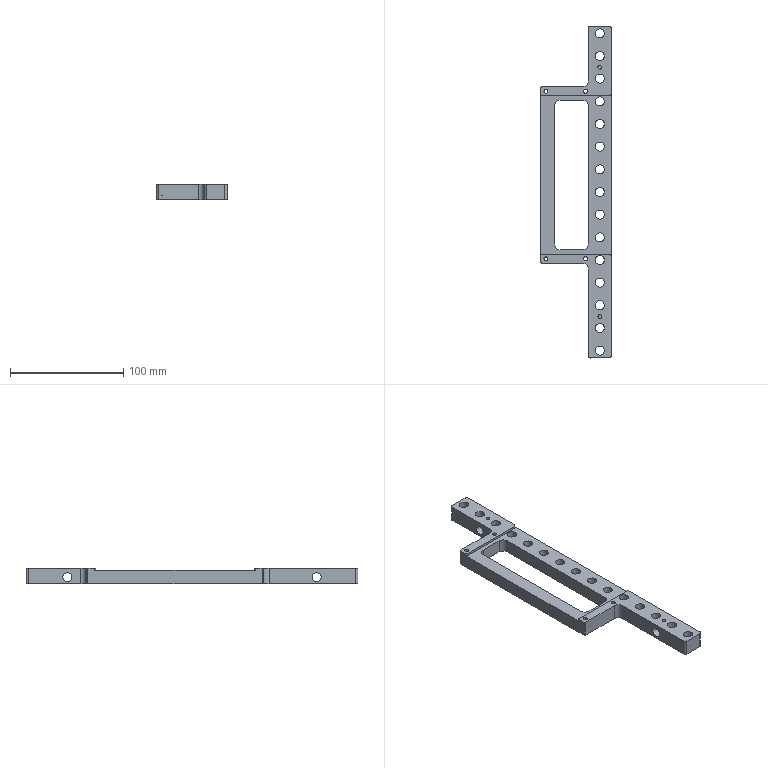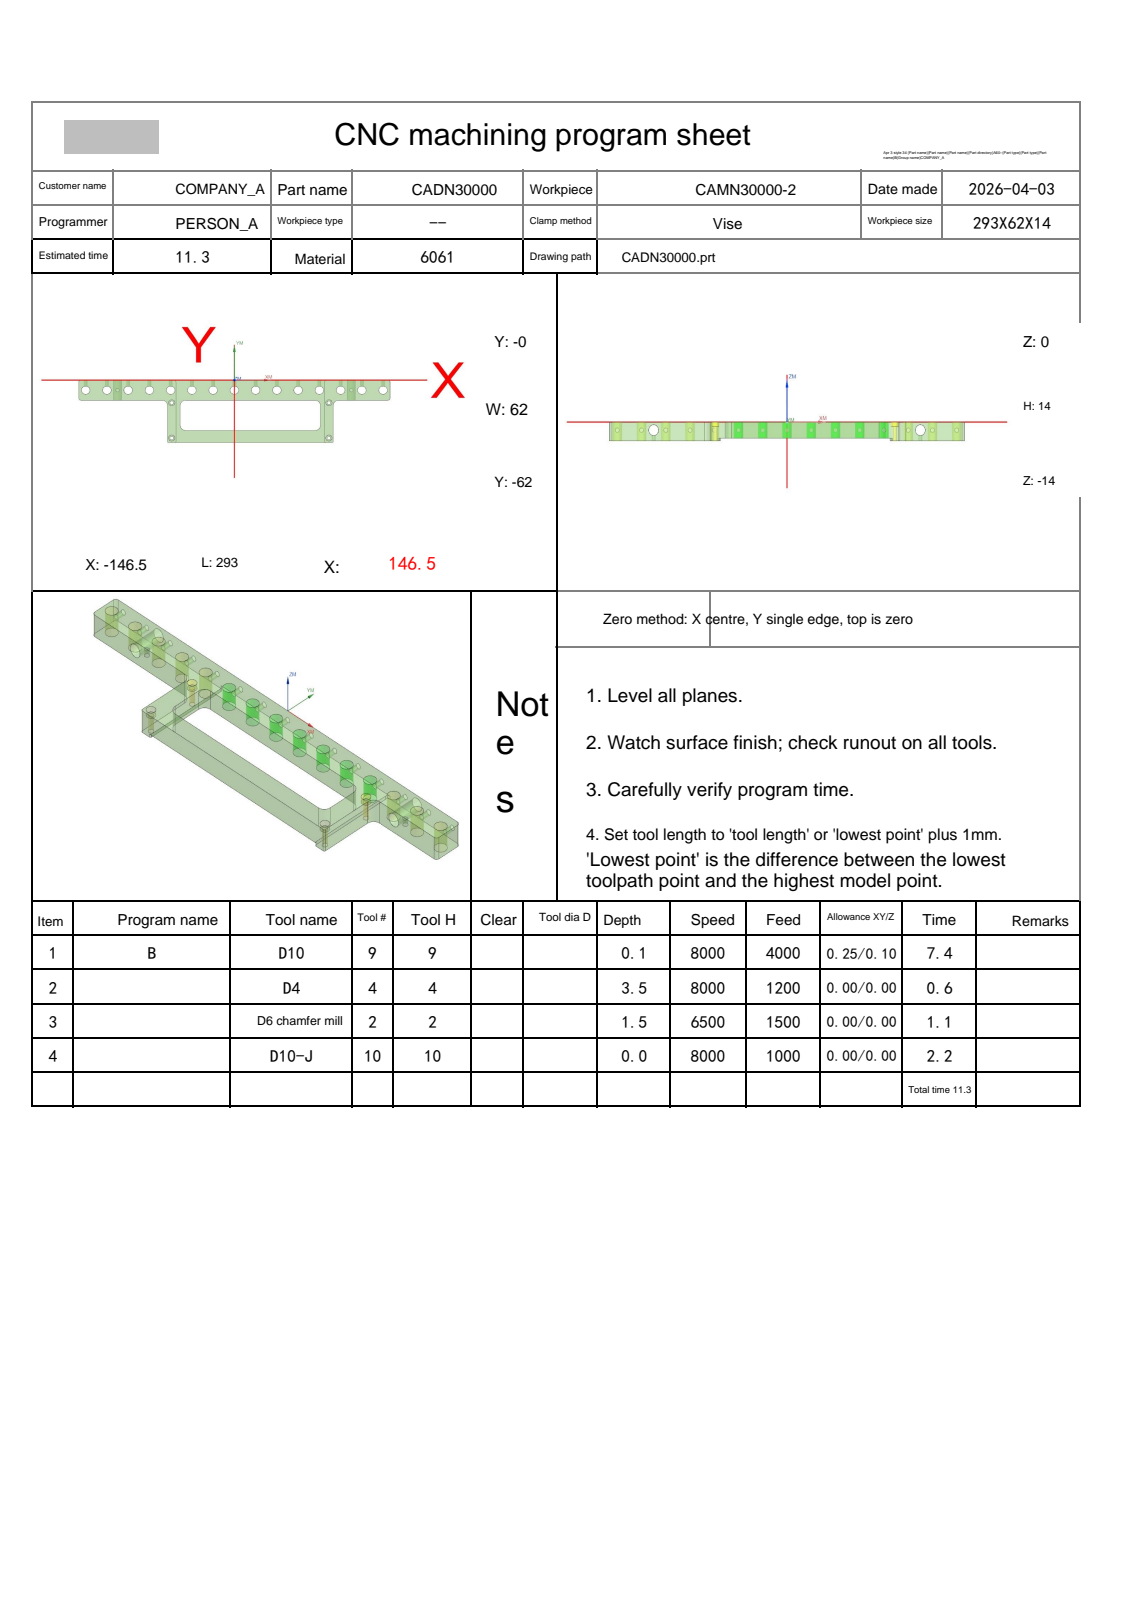NC program | NX | posted by the shop | part box 62 x 293 x 14 mm
Lines 1542 to 1949 of 1949:
N3 T02 M06
(D6 chamfer mill  D=6. R=0. H=02 ce=0.00 di=0.00)
G00 G90 G54 X-.386 Y1.227 M03 S6500
G43 H02 Z20.
M08
Z.172
G01 Z-1.499 F1500.
G03 X-.1 Y1.027 I1.286 J1.532
G01 X-.054 Y.997
X0.0 Y1.
X144.5
G02 X147.5 Y-2. I0.0 J-3.
G01 Y-18.
G02 X144.5 Y-21. I-3. J0.0
G01 X98.1
G03 X94. Y-25.1 I0.0 J-4.1
G01 Y-61.
G02 X92. Y-63. I-2. J0.0
G01 X-62.
G02 X-64. Y-61. I0.0 J2.
G01 Y-25.1
G03 X-68.1 Y-21. I-4.1 J0.0
G01 X-144.5
G02 X-147.5 Y-18. I0.0 J3.
G01 Y-2.
G02 X-144.5 Y1. I3. J0.0
G01 X0.0
X.054 Y.997
X.1 Y1.027
G03 X.386 Y1.227 I-1. J1.732
G01 Z.172
G00 Z10.
X-59.404 Y-24.308
Z.257
G01 Z-1.499
G03 X-59.102 Y-24.482 I1.147 J1.638
G01 X-59.054 Y-24.508
X-59. Y-24.5
G03 X-57. Y-22.5 I0.0 J2.
X-59. Y-20.5 I-2. J0.0
X-61. Y-22.5 I0.0 J-2.
X-59.347 Y-24.47 I2. J0.0
G01 X-59. Y-24.5
X-58.946 Y-24.508
X-58.898 Y-24.482
G03 X-58.596 Y-24.308 I-.845 J1.813
G01 Z.26
G00 Z10.
X-59.404 Y-59.308
Z.257
G01 Z-1.499
G03 X-59.102 Y-59.482 I1.147 J1.638
G01 X-59.054 Y-59.508
X-59. Y-59.5
G03 X-57. Y-57.5 I0.0 J2.
X-59. Y-55.5 I-2. J0.0
X-61. Y-57.5 I0.0 J-2.
X-59.347 Y-59.47 I2. J0.0
G01 X-59. Y-59.5
X-58.946 Y-59.508
X-58.898 Y-59.482
G03 X-58.596 Y-59.308 I-.845 J1.813
G01 Z.257
G00 Z10.
X-139.599 Y-7.147
Z.238
G01 Z-1.499
G03 X-139.898 Y-6.969 I-1.167 J-1.624
G01 X-139.946 Y-6.943
X-140. Y-6.95
G03 X-143.05 Y-10. I0.0 J-3.05
X-140. Y-13.05 I3.05 J0.0
X-136.95 Y-10. I0.0 J3.05
X-140. Y-6.95 I-3.05 J0.0
G01 X-140.054 Y-6.943
X-140.102 Y-6.969
G03 X-140.401 Y-7.147 I.868 J-1.802
G01 Z.238
G00 Z10.
X-119.599
Z.238
G01 Z-1.499
G03 X-119.898 Y-6.969 I-1.167 J-1.624
G01 X-119.946 Y-6.943
X-120. Y-6.95
G03 X-123.05 Y-10. I0.0 J-3.05
X-120. Y-13.05 I3.05 J0.0
X-116.95 Y-10. I0.0 J3.05
X-120. Y-6.95 I-3.05 J0.0
G01 X-120.054 Y-6.943
X-120.102 Y-6.969
G03 X-120.401 Y-7.147 I.868 J-1.802
G01 Z.238
G00 Z10.
X-99.599
Z.238
G01 Z-1.499
G03 X-99.898 Y-6.969 I-1.167 J-1.624
G01 X-99.946 Y-6.943
X-100. Y-6.95
G03 X-103.05 Y-10. I0.0 J-3.05
X-100. Y-13.05 I3.05 J0.0
X-96.95 Y-10. I0.0 J3.05
X-100. Y-6.95 I-3.05 J0.0
G01 X-100.054 Y-6.943
X-100.102 Y-6.969
G03 X-100.401 Y-7.147 I.868 J-1.802
G01 Z.238
G00 Z10.
X-79.599
Z.238
G01 Z-1.499
G03 X-79.898 Y-6.969 I-1.167 J-1.624
G01 X-79.946 Y-6.943
X-80. Y-6.95
G03 X-83.05 Y-10. I0.0 J-3.05
X-80. Y-13.05 I3.05 J0.0
X-76.95 Y-10. I0.0 J3.05
X-80. Y-6.95 I-3.05 J0.0
G01 X-80.054 Y-6.943
X-80.102 Y-6.969
G03 X-80.401 Y-7.147 I.868 J-1.802
G01 Z.238
G00 Z10.
X-59.599
Z.238
G01 Z-1.499
G03 X-59.898 Y-6.969 I-1.167 J-1.624
G01 X-59.946 Y-6.943
X-60. Y-6.95
G03 X-63.05 Y-10. I0.0 J-3.05
X-60. Y-13.05 I3.05 J0.0
X-56.95 Y-10. I0.0 J3.05
X-60. Y-6.95 I-3.05 J0.0
G01 X-60.054 Y-6.943
X-60.102 Y-6.969
G03 X-60.401 Y-7.147 I.868 J-1.802
G01 Z.238
G00 Z10.
X-39.599
Z.238
G01 Z-1.499
G03 X-39.898 Y-6.969 I-1.167 J-1.624
G01 X-39.946 Y-6.943
X-40. Y-6.95
G03 X-43.05 Y-10. I0.0 J-3.05
X-40. Y-13.05 I3.05 J0.0
X-36.95 Y-10. I0.0 J3.05
X-40. Y-6.95 I-3.05 J0.0
G01 X-40.054 Y-6.943
X-40.102 Y-6.969
G03 X-40.401 Y-7.147 I.868 J-1.802
G01 Z.238
G00 Z10.
X-19.599
Z.238
G01 Z-1.499
G03 X-19.898 Y-6.969 I-1.167 J-1.624
G01 X-19.946 Y-6.943
X-20. Y-6.95
G03 X-23.05 Y-10. I0.0 J-3.05
X-20. Y-13.05 I3.05 J0.0
X-16.95 Y-10. I0.0 J3.05
X-20. Y-6.95 I-3.05 J0.0
G01 X-20.054 Y-6.943
X-20.102 Y-6.969
G03 X-20.401 Y-7.147 I.868 J-1.802
G01 Z.238
G00 Z10.
X.401
Z.238
G01 Z-1.499
G03 X.102 Y-6.969 I-1.167 J-1.624
G01 X.054 Y-6.943
X0.0 Y-6.95
G03 X-3.05 Y-10. I0.0 J-3.05
X0.0 Y-13.05 I3.05 J0.0
X3.05 Y-10. I0.0 J3.05
X0.0 Y-6.95 I-3.05 J0.0
G01 X-.054 Y-6.943
X-.102 Y-6.969
G03 X-.401 Y-7.147 I.868 J-1.802
G01 Z.238
G00 Z10.
X14.614 Y-48.773
Z.172
G01 Z-1.499
G03 X14.9 Y-48.973 I1.286 J1.532
G01 X14.946 Y-49.003
X15. Y-49.
X75.9
G03 X80. Y-44.9 I0.0 J4.1
G01 Y-25.1
G03 X75.9 Y-21. I-4.1 J0.0
G01 X-45.9
G03 X-50. Y-25.1 I0.0 J-4.1
G01 Y-44.9
G03 X-45.9 Y-49. I4.1 J0.0
G01 X15.
X15.054 Y-49.003
X15.1 Y-48.973
G03 X15.386 Y-48.773 I-1. J1.732
G01 Z.172
G00 Z10.
X20.401 Y-7.147
Z.238
G01 Z-1.499
G03 X20.102 Y-6.969 I-1.167 J-1.624
G01 X20.054 Y-6.943
X20. Y-6.95
G03 X16.95 Y-10. I0.0 J-3.05
X20. Y-13.05 I3.05 J0.0
X23.05 Y-10. I0.0 J3.05
X20. Y-6.95 I-3.05 J0.0
G01 X19.946 Y-6.943
X19.898 Y-6.969
G03 X19.599 Y-7.147 I.868 J-1.802
G01 Z.238
G00 Z10.
X40.401
Z.238
G01 Z-1.499
G03 X40.102 Y-6.969 I-1.167 J-1.624
G01 X40.054 Y-6.943
X40. Y-6.95
G03 X36.95 Y-10. I0.0 J-3.05
X40. Y-13.05 I3.05 J0.0
X43.05 Y-10. I0.0 J3.05
X40. Y-6.95 I-3.05 J0.0
G01 X39.946 Y-6.943
X39.898 Y-6.969
G03 X39.599 Y-7.147 I.868 J-1.802
G01 Z.238
G00 Z10.
X60.401
Z.238
G01 Z-1.499
G03 X60.102 Y-6.969 I-1.167 J-1.624
G01 X60.054 Y-6.943
X60. Y-6.95
G03 X56.95 Y-10. I0.0 J-3.05
X60. Y-13.05 I3.05 J0.0
X63.05 Y-10. I0.0 J3.05
X60. Y-6.95 I-3.05 J0.0
G01 X59.946 Y-6.943
X59.898 Y-6.969
G03 X59.599 Y-7.147 I.868 J-1.802
G01 Z.238
G00 Z10.
X80.401
Z.238
G01 Z-1.499
G03 X80.102 Y-6.969 I-1.167 J-1.624
G01 X80.054 Y-6.943
X80. Y-6.95
G03 X76.95 Y-10. I0.0 J-3.05
X80. Y-13.05 I3.05 J0.0
X83.05 Y-10. I0.0 J3.05
X80. Y-6.95 I-3.05 J0.0
G01 X79.946 Y-6.943
X79.898 Y-6.969
G03 X79.599 Y-7.147 I.868 J-1.802
G01 Z.238
G00 Z10.
X88.596 Y-24.308
Z.257
G01 Z-1.499
G03 X88.898 Y-24.482 I1.147 J1.638
G01 X88.946 Y-24.508
X89. Y-24.5
G03 X91. Y-22.5 I0.0 J2.
X89. Y-20.5 I-2. J0.0
X87. Y-22.5 I0.0 J-2.
X88.653 Y-24.47 I2. J0.0
G01 X89. Y-24.5
X89.054 Y-24.508
X89.102 Y-24.482
G03 X89.404 Y-24.308 I-.845 J1.813
G01 Z.257
G00 Z10.
X88.596 Y-59.308
Z.257
G01 Z-1.499
G03 X88.898 Y-59.482 I1.147 J1.638
G01 X88.946 Y-59.508
X89. Y-59.5
G03 X91. Y-57.5 I0.0 J2.
X89. Y-55.5 I-2. J0.0
X87. Y-57.5 I0.0 J-2.
X88.653 Y-59.47 I2. J0.0
G01 X89. Y-59.5
X89.054 Y-59.508
X89.102 Y-59.482
G03 X89.404 Y-59.308 I-.845 J1.813
G01 Z.257
G00 Z10.
X100.401 Y-7.147
Z.238
G01 Z-1.499
G03 X100.102 Y-6.969 I-1.167 J-1.624
G01 X100.054 Y-6.943
X100. Y-6.95
G03 X96.95 Y-10. I0.0 J-3.05
X100. Y-13.05 I3.05 J0.0
X103.05 Y-10. I0.0 J3.05
X100. Y-6.95 I-3.05 J0.0
G01 X99.946 Y-6.943
X99.898 Y-6.969
G03 X99.599 Y-7.147 I.868 J-1.802
G01 Z.238
G00 Z10.
X120.401
Z.238
G01 Z-1.499
G03 X120.102 Y-6.969 I-1.167 J-1.624
G01 X120.054 Y-6.943
X120. Y-6.95
G03 X116.95 Y-10. I0.0 J-3.05
X120. Y-13.05 I3.05 J0.0
X123.05 Y-10. I0.0 J3.05
X120. Y-6.95 I-3.05 J0.0
G01 X119.946 Y-6.943
X119.898 Y-6.969
G03 X119.599 Y-7.147 I.868 J-1.802
G01 Z.238
G00 Z10.
X140.401
Z.238
G01 Z-1.499
G03 X140.102 Y-6.969 I-1.167 J-1.624
G01 X140.054 Y-6.943
X140. Y-6.95
G03 X136.95 Y-10. I0.0 J-3.05
X140. Y-13.05 I3.05 J0.0
X143.05 Y-10. I0.0 J3.05
X140. Y-6.95 I-3.05 J0.0
G01 X139.946 Y-6.943
X139.898 Y-6.969
G03 X139.599 Y-7.147 I.868 J-1.802
G01 Z.238
G00 Z20.
G91 G28 Z0.0
M05
M09
G91 G28 Z0.0
M01
N4 T10 M06
(D10-J  D=10. R=0. H=10 ce=0.00 di=0.00)
G00 G90 G54 X-163.499 Y-3.202 M03 S8000
G43 H10 Z20.
M08
Z2.
G01 Z0.0 F1000.
X-151.499 Y-3.049
X150.209 Y.806
X150.221
G02 X151.174 Y.108 I0.0 J-1.
X151.499 Y-2. I-6.674 J-2.108
G01 Y-5.449
G02 X150.513 Y-6.448 I-1. J.001
G01 X-150.513 Y-10.294
G03 X-151.499 Y-11.293 I.014 J-1.
G01 Y-16.654
G03 X-150.599 Y-17.553 I.9 J.001
G01 X-150.589
X150.589 Y-13.705
X150.599
G02 X151.499 Y-14.604 I0.0 J-.9
G01 Y-18.
G02 X151.111 Y-20.297 I-6.999 J0.0
X150.181 Y-20.968 I-.944 J.329
G01 X-146.329 Y-24.756
X-145.77 Y-24.881
X-145.684 Y-24.896
X-145.142 Y-24.968
X-145.09 Y-24.974
X-68.043 Y-31.009
X-67.955 Y-31.012
X97.088 Y-28.903
X97.099
G02 X97.999 Y-29.803 I0.0 J-.9
G01 Y-35.163
G02 X97.013 Y-36.162 I-1. J.001
G01 X-67.013 Y-38.258
G03 X-67.999 Y-39.257 I.014 J-1.
G01 Y-44.617
G03 X-67.099 Y-45.516 I.9 J.001
G01 X-67.088
X97.088 Y-43.419
X97.099
G02 X97.999 Y-44.318 I0.0 J-.9
G01 Y-49.678
G02 X97.013 Y-50.677 I-1. J.001
G01 X-67.013 Y-52.773
G03 X-67.999 Y-53.772 I.014 J-1.
G01 Y-59.132
G03 X-67.099 Y-60.031 I.9 J.001
G01 X-67.088
X97.999 Y-57.922
X109.999 Y-57.769
Z2.
G00 Z20.
M05
M09
G91 G28 Z0.0
G91 G28 Y0.0
M30
%